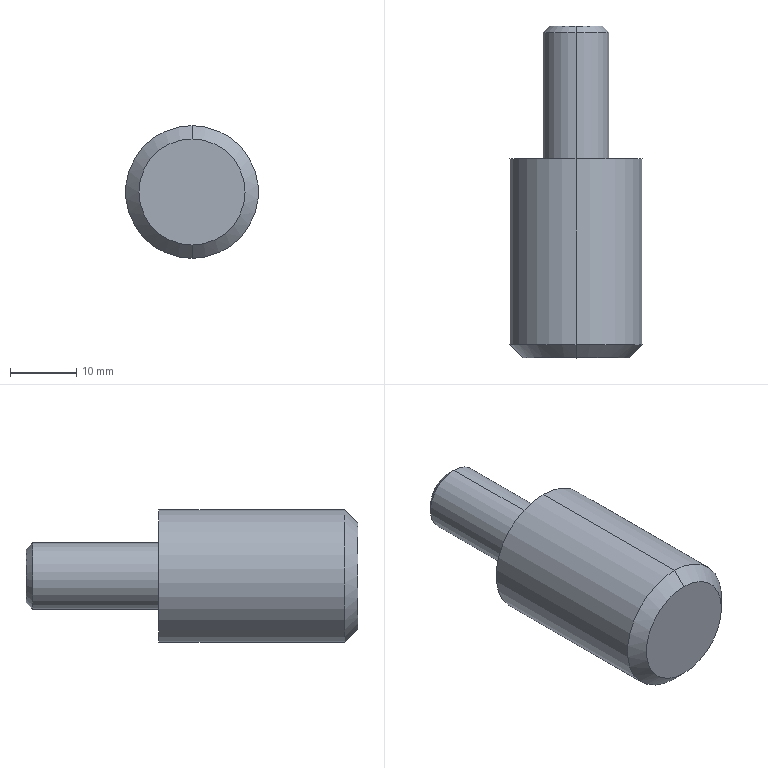Part | SolidWorks | features Chamfer 2, Extrusion 1, ICE 1 | 1 solid | 11 faces | box 20 x 50 x 20 mm | volume 10864 mm3 | cone 4 | cylinder 4 | plane 3 | commonest cylinder face diameters 10 x2 20 x2
STEP:
#1=CARTESIAN_POINT('',(0.,50.,4.));
#2=VERTEX_POINT('',#1);
#3=CARTESIAN_POINT('',(0.,50.,-4.));
#4=VERTEX_POINT('',#3);
#5=CARTESIAN_POINT('',(0.,50.,0.));
#6=DIRECTION('',(0.,1.,0.));
#7=DIRECTION('',(0.,0.,1.));
#8=AXIS2_PLACEMENT_3D('',#5,#6,#7);
#9=CIRCLE('',#8,4.);
#10=EDGE_CURVE('',#2,#4,#9,.T.);
#11=ORIENTED_EDGE('',*,*,#10,.F.);
#12=CARTESIAN_POINT('',(0.,49.,5.));
#13=VERTEX_POINT('',#12);
#14=CARTESIAN_POINT('',(0.,50.,4.));
#15=DIRECTION('',(0.,-0.7071,0.7071));
#16=VECTOR('',#15,1000.);
#17=LINE('',#14,#16);
#18=EDGE_CURVE('',#2,#13,#17,.T.);
#19=ORIENTED_EDGE('',*,*,#18,.T.);
#20=CARTESIAN_POINT('',(0.,49.,-5.));
#21=VERTEX_POINT('',#20);
#22=CARTESIAN_POINT('',(0.,49.,0.));
#23=DIRECTION('',(0.,-1.,0.));
#24=DIRECTION('',(0.,0.,1.));
#25=AXIS2_PLACEMENT_3D('',#22,#23,#24);
#26=CIRCLE('',#25,5.);
#27=EDGE_CURVE('',#21,#13,#26,.T.);
#28=ORIENTED_EDGE('',*,*,#27,.F.);
#29=CARTESIAN_POINT('',(0.,50.,-4.));
#30=DIRECTION('',(0.,-0.7071,-0.7071));
#31=VECTOR('',#30,1000.);
#32=LINE('',#29,#31);
#33=EDGE_CURVE('',#4,#21,#32,.T.);
#34=ORIENTED_EDGE('',*,*,#33,.F.);
#35=EDGE_LOOP('',(#11,#19,#28,#34));
#36=FACE_OUTER_BOUND('',#35,.T.);
#37=CARTESIAN_POINT('',(0.,50.,0.));
#38=DIRECTION('',(0.,-1.,0.));
#39=DIRECTION('',(0.,0.,-1.));
#40=AXIS2_PLACEMENT_3D('',#37,#38,#39);
#41=CONICAL_SURFACE('',#40,4.,0.7854);
#42=ADVANCED_FACE('',(#36),#41,.T.);
#43=CARTESIAN_POINT('',(0.,0.,-8.));
#44=VERTEX_POINT('',#43);
#45=CARTESIAN_POINT('',(0.,0.,8.));
#46=VERTEX_POINT('',#45);
#47=CARTESIAN_POINT('',(0.,0.,0.));
#48=DIRECTION('',(0.,-1.,0.));
#49=DIRECTION('',(0.,0.,1.));
#50=AXIS2_PLACEMENT_3D('',#47,#48,#49);
#51=CIRCLE('',#50,8.);
#52=EDGE_CURVE('',#44,#46,#51,.T.);
#53=ORIENTED_EDGE('',*,*,#52,.F.);
#54=CARTESIAN_POINT('',(0.,2.,-10.));
#55=VERTEX_POINT('',#54);
#56=CARTESIAN_POINT('',(0.,2.,-10.));
#57=DIRECTION('',(0.,0.7071,-0.7071));
#58=VECTOR('',#57,1000.);
#59=LINE('',#56,#58);
#60=EDGE_CURVE('',#44,#55,#59,.T.);
#61=ORIENTED_EDGE('',*,*,#60,.T.);
#62=CARTESIAN_POINT('',(0.,2.,10.));
#63=VERTEX_POINT('',#62);
#64=CARTESIAN_POINT('',(0.,2.,0.));
#65=DIRECTION('',(0.,1.,0.));
#66=DIRECTION('',(0.,0.,1.));
#67=AXIS2_PLACEMENT_3D('',#64,#65,#66);
#68=CIRCLE('',#67,10.);
#69=EDGE_CURVE('',#63,#55,#68,.T.);
#70=ORIENTED_EDGE('',*,*,#69,.F.);
#71=CARTESIAN_POINT('',(0.,2.,10.));
#72=DIRECTION('',(0.,0.7071,0.7071));
#73=VECTOR('',#72,1000.);
#74=LINE('',#71,#73);
#75=EDGE_CURVE('',#46,#63,#74,.T.);
#76=ORIENTED_EDGE('',*,*,#75,.F.);
#77=EDGE_LOOP('',(#53,#61,#70,#76));
#78=FACE_OUTER_BOUND('',#77,.T.);
#79=CARTESIAN_POINT('',(0.,2.,0.));
#80=DIRECTION('',(0.,1.,0.));
#81=DIRECTION('',(0.,0.,1.));
#82=AXIS2_PLACEMENT_3D('',#79,#80,#81);
#83=CONICAL_SURFACE('',#82,10.,0.7854);
#84=ADVANCED_FACE('',(#78),#83,.T.);
#85=ORIENTED_EDGE('',*,*,#27,.T.);
#86=CARTESIAN_POINT('',(0.,30.,5.));
#87=VERTEX_POINT('',#86);
#88=CARTESIAN_POINT('',(0.,50.,5.));
#89=DIRECTION('',(0.,-1.,0.));
#90=VECTOR('',#89,1000.);
#91=LINE('',#88,#90);
#92=EDGE_CURVE('',#13,#87,#91,.T.);
#93=ORIENTED_EDGE('',*,*,#92,.T.);
#94=CARTESIAN_POINT('',(0.,30.,-5.));
#95=VERTEX_POINT('',#94);
#96=CARTESIAN_POINT('',(0.,30.,0.));
#97=DIRECTION('',(0.,1.,0.));
#98=DIRECTION('',(0.,0.,1.));
#99=AXIS2_PLACEMENT_3D('',#96,#97,#98);
#100=CIRCLE('',#99,5.);
#101=EDGE_CURVE('',#87,#95,#100,.T.);
#102=ORIENTED_EDGE('',*,*,#101,.T.);
#103=CARTESIAN_POINT('',(0.,50.,-5.));
#104=DIRECTION('',(0.,-1.,0.));
#105=VECTOR('',#104,1000.);
#106=LINE('',#103,#105);
#107=EDGE_CURVE('',#21,#95,#106,.T.);
#108=ORIENTED_EDGE('',*,*,#107,.F.);
#109=EDGE_LOOP('',(#85,#93,#102,#108));
#110=FACE_OUTER_BOUND('',#109,.T.);
#111=CARTESIAN_POINT('',(0.,50.,0.));
#112=DIRECTION('',(0.,-1.,0.));
#113=DIRECTION('',(0.,0.,-1.));
#114=AXIS2_PLACEMENT_3D('',#111,#112,#113);
#115=CYLINDRICAL_SURFACE('',#114,5.);
#116=ADVANCED_FACE('',(#110),#115,.T.);
#117=CARTESIAN_POINT('',(0.,30.,10.));
#118=VERTEX_POINT('',#117);
#119=CARTESIAN_POINT('',(0.,30.,-10.));
#120=VERTEX_POINT('',#119);
#121=CARTESIAN_POINT('',(0.,30.,0.));
#122=DIRECTION('',(0.,1.,0.));
#123=DIRECTION('',(0.,0.,1.));
#124=AXIS2_PLACEMENT_3D('',#121,#122,#123);
#125=CIRCLE('',#124,10.);
#126=EDGE_CURVE('',#118,#120,#125,.T.);
#127=ORIENTED_EDGE('',*,*,#126,.F.);
#128=CARTESIAN_POINT('',(0.,30.,10.));
#129=DIRECTION('',(0.,-1.,0.));
#130=VECTOR('',#129,1000.);
#131=LINE('',#128,#130);
#132=EDGE_CURVE('',#118,#63,#131,.T.);
#133=ORIENTED_EDGE('',*,*,#132,.T.);
#134=ORIENTED_EDGE('',*,*,#69,.T.);
#135=CARTESIAN_POINT('',(0.,30.,-10.));
#136=DIRECTION('',(0.,-1.,0.));
#137=VECTOR('',#136,1000.);
#138=LINE('',#135,#137);
#139=EDGE_CURVE('',#120,#55,#138,.T.);
#140=ORIENTED_EDGE('',*,*,#139,.F.);
#141=EDGE_LOOP('',(#127,#133,#134,#140));
#142=FACE_OUTER_BOUND('',#141,.T.);
#143=CARTESIAN_POINT('',(0.,30.,0.));
#144=DIRECTION('',(0.,-1.,0.));
#145=DIRECTION('',(0.,0.,-1.));
#146=AXIS2_PLACEMENT_3D('',#143,#144,#145);
#147=CYLINDRICAL_SURFACE('',#146,10.);
#148=ADVANCED_FACE('',(#142),#147,.T.);
#149=ORIENTED_EDGE('',*,*,#132,.F.);
#150=CARTESIAN_POINT('',(0.,30.,0.));
#151=DIRECTION('',(0.,1.,0.));
#152=DIRECTION('',(0.,0.,1.));
#153=AXIS2_PLACEMENT_3D('',#150,#151,#152);
#154=CIRCLE('',#153,10.);
#155=EDGE_CURVE('',#120,#118,#154,.T.);
#156=ORIENTED_EDGE('',*,*,#155,.F.);
#157=ORIENTED_EDGE('',*,*,#139,.T.);
#158=CARTESIAN_POINT('',(0.,2.,0.));
#159=DIRECTION('',(0.,1.,0.));
#160=DIRECTION('',(0.,0.,1.));
#161=AXIS2_PLACEMENT_3D('',#158,#159,#160);
#162=CIRCLE('',#161,10.);
#163=EDGE_CURVE('',#55,#63,#162,.T.);
#164=ORIENTED_EDGE('',*,*,#163,.T.);
#165=EDGE_LOOP('',(#149,#156,#157,#164));
#166=FACE_OUTER_BOUND('',#165,.T.);
#167=CARTESIAN_POINT('',(0.,30.,0.));
#168=DIRECTION('',(0.,-1.,0.));
#169=DIRECTION('',(0.,0.,-1.));
#170=AXIS2_PLACEMENT_3D('',#167,#168,#169);
#171=CYLINDRICAL_SURFACE('',#170,10.);
#172=ADVANCED_FACE('',(#166),#171,.T.);
#173=CARTESIAN_POINT('',(0.,30.,0.));
#174=DIRECTION('',(0.,1.,0.));
#175=DIRECTION('',(0.,0.,1.));
#176=AXIS2_PLACEMENT_3D('',#173,#174,#175);
#177=CIRCLE('',#176,5.);
#178=EDGE_CURVE('',#95,#87,#177,.T.);
#179=ORIENTED_EDGE('',*,*,#178,.F.);
#180=ORIENTED_EDGE('',*,*,#101,.F.);
#181=EDGE_LOOP('',(#179,#180));
#182=FACE_BOUND('',#181,.T.);
#183=ORIENTED_EDGE('',*,*,#155,.T.);
#184=ORIENTED_EDGE('',*,*,#126,.T.);
#185=EDGE_LOOP('',(#183,#184));
#186=FACE_OUTER_BOUND('',#185,.T.);
#187=CARTESIAN_POINT('',(0.,30.,0.));
#188=DIRECTION('',(0.,1.,0.));
#189=DIRECTION('',(0.,0.,1.));
#190=AXIS2_PLACEMENT_3D('',#187,#188,#189);
#191=PLANE('',#190);
#192=ADVANCED_FACE('',(#182,#186),#191,.T.);
#193=CARTESIAN_POINT('',(0.,0.,0.));
#194=DIRECTION('',(0.,-1.,0.));
#195=DIRECTION('',(0.,0.,1.));
#196=AXIS2_PLACEMENT_3D('',#193,#194,#195);
#197=CIRCLE('',#196,8.);
#198=EDGE_CURVE('',#46,#44,#197,.T.);
#199=ORIENTED_EDGE('',*,*,#198,.T.);
#200=ORIENTED_EDGE('',*,*,#52,.T.);
#201=EDGE_LOOP('',(#199,#200));
#202=FACE_OUTER_BOUND('',#201,.T.);
#203=CARTESIAN_POINT('',(0.,0.,0.));
#204=DIRECTION('',(0.,1.,0.));
#205=DIRECTION('',(0.,0.,1.));
#206=AXIS2_PLACEMENT_3D('',#203,#204,#205);
#207=PLANE('',#206);
#208=ADVANCED_FACE('',(#202),#207,.F.);
#209=ORIENTED_EDGE('',*,*,#92,.F.);
#210=CARTESIAN_POINT('',(0.,49.,0.));
#211=DIRECTION('',(0.,-1.,0.));
#212=DIRECTION('',(0.,0.,1.));
#213=AXIS2_PLACEMENT_3D('',#210,#211,#212);
#214=CIRCLE('',#213,5.);
#215=EDGE_CURVE('',#13,#21,#214,.T.);
#216=ORIENTED_EDGE('',*,*,#215,.T.);
#217=ORIENTED_EDGE('',*,*,#107,.T.);
#218=ORIENTED_EDGE('',*,*,#178,.T.);
#219=EDGE_LOOP('',(#209,#216,#217,#218));
#220=FACE_OUTER_BOUND('',#219,.T.);
#221=CARTESIAN_POINT('',(0.,50.,0.));
#222=DIRECTION('',(0.,-1.,0.));
#223=DIRECTION('',(0.,0.,-1.));
#224=AXIS2_PLACEMENT_3D('',#221,#222,#223);
#225=CYLINDRICAL_SURFACE('',#224,5.);
#226=ADVANCED_FACE('',(#220),#225,.T.);
#227=CARTESIAN_POINT('',(0.,50.,0.));
#228=DIRECTION('',(0.,1.,0.));
#229=DIRECTION('',(0.,0.,1.));
#230=AXIS2_PLACEMENT_3D('',#227,#228,#229);
#231=CIRCLE('',#230,4.);
#232=EDGE_CURVE('',#4,#2,#231,.T.);
#233=ORIENTED_EDGE('',*,*,#232,.T.);
#234=ORIENTED_EDGE('',*,*,#10,.T.);
#235=EDGE_LOOP('',(#233,#234));
#236=FACE_OUTER_BOUND('',#235,.T.);
#237=CARTESIAN_POINT('',(0.,50.,0.));
#238=DIRECTION('',(0.,1.,0.));
#239=DIRECTION('',(0.,0.,1.));
#240=AXIS2_PLACEMENT_3D('',#237,#238,#239);
#241=PLANE('',#240);
#242=ADVANCED_FACE('',(#236),#241,.T.);
#243=ORIENTED_EDGE('',*,*,#60,.F.);
#244=ORIENTED_EDGE('',*,*,#198,.F.);
#245=ORIENTED_EDGE('',*,*,#75,.T.);
#246=ORIENTED_EDGE('',*,*,#163,.F.);
#247=EDGE_LOOP('',(#243,#244,#245,#246));
#248=FACE_OUTER_BOUND('',#247,.T.);
#249=CARTESIAN_POINT('',(0.,2.,0.));
#250=DIRECTION('',(0.,1.,0.));
#251=DIRECTION('',(0.,0.,1.));
#252=AXIS2_PLACEMENT_3D('',#249,#250,#251);
#253=CONICAL_SURFACE('',#252,10.,0.7854);
#254=ADVANCED_FACE('',(#248),#253,.T.);
#255=ORIENTED_EDGE('',*,*,#18,.F.);
#256=ORIENTED_EDGE('',*,*,#232,.F.);
#257=ORIENTED_EDGE('',*,*,#33,.T.);
#258=ORIENTED_EDGE('',*,*,#215,.F.);
#259=EDGE_LOOP('',(#255,#256,#257,#258));
#260=FACE_OUTER_BOUND('',#259,.T.);
#261=CARTESIAN_POINT('',(0.,50.,0.));
#262=DIRECTION('',(0.,-1.,0.));
#263=DIRECTION('',(0.,0.,-1.));
#264=AXIS2_PLACEMENT_3D('',#261,#262,#263);
#265=CONICAL_SURFACE('',#264,4.,0.7854);
#266=ADVANCED_FACE('',(#260),#265,.T.);
#267=CLOSED_SHELL('',(#42,#84,#116,#148,#172,#192,#208,#226,#242,#254,#266));
#268=MANIFOLD_SOLID_BREP('',#267);
#269=CARTESIAN_POINT('',(0.,0.,0.));
#270=DIRECTION('',(0.,0.,1.));
#271=DIRECTION('',(1.,0.,0.));
#272=AXIS2_PLACEMENT_3D('',#269,#270,#271);
#273=(LENGTH_UNIT()NAMED_UNIT(*)SI_UNIT(.MILLI.,.METRE.));
#274=UNCERTAINTY_MEASURE_WITH_UNIT(LENGTH_MEASURE(0.00001),#273,'','');
#275=(NAMED_UNIT(*)PLANE_ANGLE_UNIT()SI_UNIT($,.RADIAN.));
#276=(NAMED_UNIT(*)SI_UNIT($,.STERADIAN.)SOLID_ANGLE_UNIT());
#277=(GEOMETRIC_REPRESENTATION_CONTEXT(3)GLOBAL_UNCERTAINTY_ASSIGNED_CONTEXT((#274))GLOBAL_UNIT_ASSIGNED_CONTEXT((#273,#275,#276))REPRESENTATION_CONTEXT('',''));
#278=ADVANCED_BREP_SHAPE_REPRESENTATION('',(#268,#272),#277);